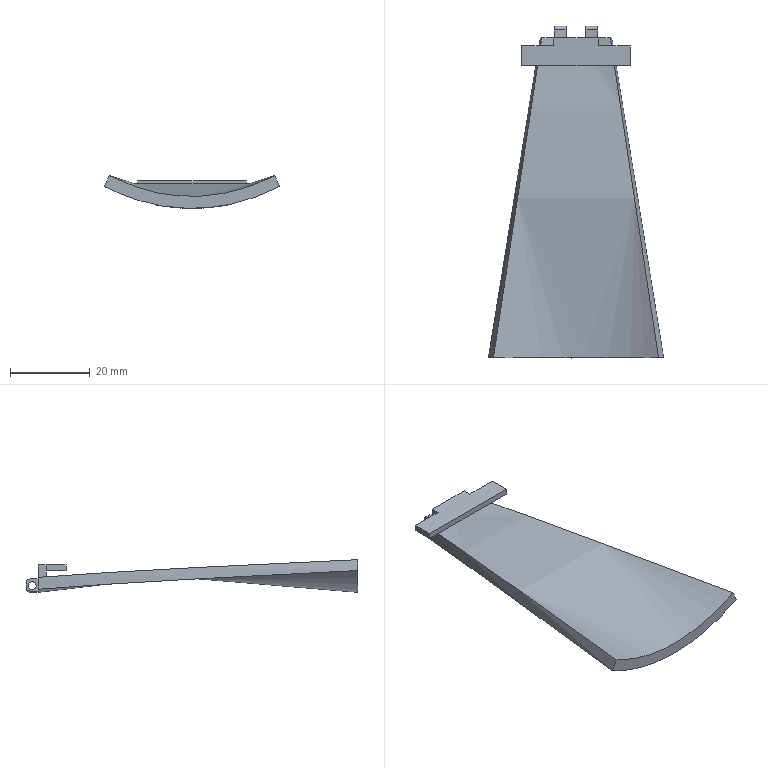Part | SolidWorks | features ICE 6, MoveFace 6, Blend 1, Fillet 1 | 1 solid | 34 faces | box 43.809 x 83 x 8.178 mm | volume 7265 mm3 | plane 18 | cylinder 8 | spline 4 | torus 4 | commonest cylinder face diameters 2 x4 86 x2 92 x2
STEP:
#1=CARTESIAN_POINT('',(-5.5,81.49,-43.311));
#2=VERTEX_POINT('',#1);
#3=CARTESIAN_POINT('',(-5.5,81.49,-45.311));
#4=VERTEX_POINT('',#3);
#5=CARTESIAN_POINT('',(-5.5,81.49,-44.311));
#6=DIRECTION('',(1.,0.,0.));
#7=DIRECTION('',(0.,0.,-1.));
#8=AXIS2_PLACEMENT_3D('',#5,#6,#7);
#9=CIRCLE('',#8,1.);
#10=EDGE_CURVE('',#2,#4,#9,.T.);
#11=ORIENTED_EDGE('',*,*,#10,.F.);
#12=CARTESIAN_POINT('',(-2.5,81.49,-43.311));
#13=VERTEX_POINT('',#12);
#14=CARTESIAN_POINT('',(-6.,81.49,-43.311));
#15=DIRECTION('',(1.,0.,0.));
#16=VECTOR('',#15,1000.);
#17=LINE('',#14,#16);
#18=EDGE_CURVE('',#2,#13,#17,.T.);
#19=ORIENTED_EDGE('',*,*,#18,.T.);
#20=CARTESIAN_POINT('',(-2.5,81.49,-45.311));
#21=VERTEX_POINT('',#20);
#22=CARTESIAN_POINT('',(-2.5,81.49,-44.311));
#23=DIRECTION('',(1.,0.,0.));
#24=DIRECTION('',(0.,0.,-1.));
#25=AXIS2_PLACEMENT_3D('',#22,#23,#24);
#26=CIRCLE('',#25,1.);
#27=EDGE_CURVE('',#13,#21,#26,.T.);
#28=ORIENTED_EDGE('',*,*,#27,.T.);
#29=CARTESIAN_POINT('',(-6.,81.49,-45.311));
#30=DIRECTION('',(1.,0.,0.));
#31=VECTOR('',#30,1000.);
#32=LINE('',#29,#31);
#33=EDGE_CURVE('',#4,#21,#32,.T.);
#34=ORIENTED_EDGE('',*,*,#33,.F.);
#35=EDGE_LOOP('',(#11,#19,#28,#34));
#36=FACE_OUTER_BOUND('',#35,.T.);
#37=CARTESIAN_POINT('',(-6.,81.49,-44.311));
#38=DIRECTION('',(1.,0.,0.));
#39=DIRECTION('',(0.,0.,-1.));
#40=AXIS2_PLACEMENT_3D('',#37,#38,#39);
#41=CYLINDRICAL_SURFACE('',#40,1.);
#42=ADVANCED_FACE('',(#36),#41,.F.);
#43=CARTESIAN_POINT('',(2.5,81.49,-45.311));
#44=VERTEX_POINT('',#43);
#45=CARTESIAN_POINT('',(2.5,81.49,-43.311));
#46=VERTEX_POINT('',#45);
#47=CARTESIAN_POINT('',(2.5,81.49,-44.311));
#48=DIRECTION('',(-1.,0.,0.));
#49=DIRECTION('',(0.,0.,1.));
#50=AXIS2_PLACEMENT_3D('',#47,#48,#49);
#51=CIRCLE('',#50,1.);
#52=EDGE_CURVE('',#44,#46,#51,.T.);
#53=ORIENTED_EDGE('',*,*,#52,.T.);
#54=CARTESIAN_POINT('',(5.5,81.49,-43.311));
#55=VERTEX_POINT('',#54);
#56=CARTESIAN_POINT('',(-6.,81.49,-43.311));
#57=DIRECTION('',(1.,0.,0.));
#58=VECTOR('',#57,1000.);
#59=LINE('',#56,#58);
#60=EDGE_CURVE('',#46,#55,#59,.T.);
#61=ORIENTED_EDGE('',*,*,#60,.T.);
#62=CARTESIAN_POINT('',(5.5,81.49,-45.311));
#63=VERTEX_POINT('',#62);
#64=CARTESIAN_POINT('',(5.5,81.49,-44.311));
#65=DIRECTION('',(1.,0.,0.));
#66=DIRECTION('',(0.,0.,-1.));
#67=AXIS2_PLACEMENT_3D('',#64,#65,#66);
#68=CIRCLE('',#67,1.);
#69=EDGE_CURVE('',#55,#63,#68,.T.);
#70=ORIENTED_EDGE('',*,*,#69,.T.);
#71=CARTESIAN_POINT('',(-6.,81.49,-45.311));
#72=DIRECTION('',(1.,0.,0.));
#73=VECTOR('',#72,1000.);
#74=LINE('',#71,#73);
#75=EDGE_CURVE('',#44,#63,#74,.T.);
#76=ORIENTED_EDGE('',*,*,#75,.F.);
#77=EDGE_LOOP('',(#53,#61,#70,#76));
#78=FACE_OUTER_BOUND('',#77,.T.);
#79=CARTESIAN_POINT('',(-6.,81.49,-44.311));
#80=DIRECTION('',(1.,0.,0.));
#81=DIRECTION('',(0.,0.,-1.));
#82=AXIS2_PLACEMENT_3D('',#79,#80,#81);
#83=CYLINDRICAL_SURFACE('',#82,1.);
#84=ADVANCED_FACE('',(#78),#83,.F.);
#85=CARTESIAN_POINT('',(-5.613,78.,-42.588));
#86=VERTEX_POINT('',#85);
#87=CARTESIAN_POINT('',(-5.613,78.,-40.632));
#88=VERTEX_POINT('',#87);
#89=CARTESIAN_POINT('',(-5.613,78.,-39.632));
#90=DIRECTION('',(0.,0.,1.));
#91=VECTOR('',#90,1000.);
#92=LINE('',#89,#91);
#93=EDGE_CURVE('',#86,#88,#92,.T.);
#94=ORIENTED_EDGE('',*,*,#93,.T.);
#95=CARTESIAN_POINT('',(-5.613,78.,-39.132));
#96=VERTEX_POINT('',#95);
#97=CARTESIAN_POINT('',(-5.613,78.,-38.132));
#98=DIRECTION('',(0.,0.,-1.));
#99=VECTOR('',#98,1000.);
#100=LINE('',#97,#99);
#101=EDGE_CURVE('',#96,#88,#100,.T.);
#102=ORIENTED_EDGE('',*,*,#101,.F.);
#103=CARTESIAN_POINT('',(-5.613,80.,-39.132));
#104=VERTEX_POINT('',#103);
#105=CARTESIAN_POINT('',(-5.613,78.,-39.132));
#106=DIRECTION('',(0.,1.,0.));
#107=VECTOR('',#106,1000.);
#108=LINE('',#105,#107);
#109=EDGE_CURVE('',#96,#104,#108,.T.);
#110=ORIENTED_EDGE('',*,*,#109,.T.);
#111=CARTESIAN_POINT('',(-5.613,80.,-42.632));
#112=VERTEX_POINT('',#111);
#113=CARTESIAN_POINT('',(-5.613,80.,-39.632));
#114=DIRECTION('',(0.,0.,1.));
#115=VECTOR('',#114,1000.);
#116=LINE('',#113,#115);
#117=EDGE_CURVE('',#112,#104,#116,.T.);
#118=ORIENTED_EDGE('',*,*,#117,.F.);
#119=CARTESIAN_POINT('',(-5.613,80.,-42.632));
#120=CARTESIAN_POINT('',(-5.613,79.333,-42.615));
#121=CARTESIAN_POINT('',(-5.613,78.667,-42.601));
#122=CARTESIAN_POINT('',(-5.613,78.,-42.588));
#123=B_SPLINE_CURVE_WITH_KNOTS('',3,(#119,#120,#121,#122),.UNSPECIFIED.,.F.,.F.,(4,4),(0.01005,0.01205),.UNSPECIFIED.);
#124=EDGE_CURVE('',#112,#86,#123,.T.);
#125=ORIENTED_EDGE('',*,*,#124,.T.);
#126=EDGE_LOOP('',(#94,#102,#110,#118,#125));
#127=FACE_OUTER_BOUND('',#126,.T.);
#128=CARTESIAN_POINT('',(-5.613,78.,-39.632));
#129=DIRECTION('',(-1.,0.,0.));
#130=DIRECTION('',(0.,0.,1.));
#131=AXIS2_PLACEMENT_3D('',#128,#129,#130);
#132=PLANE('',#131);
#133=ADVANCED_FACE('',(#127),#132,.T.);
#134=CARTESIAN_POINT('',(5.613,78.,-39.132));
#135=VERTEX_POINT('',#134);
#136=CARTESIAN_POINT('',(5.613,80.,-39.132));
#137=VERTEX_POINT('',#136);
#138=CARTESIAN_POINT('',(5.613,78.,-39.132));
#139=DIRECTION('',(0.,1.,0.));
#140=VECTOR('',#139,1000.);
#141=LINE('',#138,#140);
#142=EDGE_CURVE('',#135,#137,#141,.T.);
#143=ORIENTED_EDGE('',*,*,#142,.F.);
#144=CARTESIAN_POINT('',(5.613,78.,-40.632));
#145=VERTEX_POINT('',#144);
#146=CARTESIAN_POINT('',(5.613,78.,-38.132));
#147=DIRECTION('',(0.,0.,1.));
#148=VECTOR('',#147,1000.);
#149=LINE('',#146,#148);
#150=EDGE_CURVE('',#145,#135,#149,.T.);
#151=ORIENTED_EDGE('',*,*,#150,.F.);
#152=CARTESIAN_POINT('',(5.613,78.,-42.588));
#153=VERTEX_POINT('',#152);
#154=CARTESIAN_POINT('',(5.613,78.,-36.632));
#155=DIRECTION('',(0.,0.,-1.));
#156=VECTOR('',#155,1000.);
#157=LINE('',#154,#156);
#158=EDGE_CURVE('',#145,#153,#157,.T.);
#159=ORIENTED_EDGE('',*,*,#158,.T.);
#160=CARTESIAN_POINT('',(5.613,80.,-42.632));
#161=VERTEX_POINT('',#160);
#162=CARTESIAN_POINT('',(5.613,78.,-42.588));
#163=CARTESIAN_POINT('',(5.613,78.667,-42.601));
#164=CARTESIAN_POINT('',(5.613,79.333,-42.615));
#165=CARTESIAN_POINT('',(5.613,80.,-42.632));
#166=B_SPLINE_CURVE_WITH_KNOTS('',3,(#162,#163,#164,#165),.UNSPECIFIED.,.F.,.F.,(4,4),(0.01205,0.01405),.UNSPECIFIED.);
#167=EDGE_CURVE('',#153,#161,#166,.T.);
#168=ORIENTED_EDGE('',*,*,#167,.T.);
#169=CARTESIAN_POINT('',(5.613,80.,-36.632));
#170=DIRECTION('',(0.,0.,-1.));
#171=VECTOR('',#170,1000.);
#172=LINE('',#169,#171);
#173=EDGE_CURVE('',#137,#161,#172,.T.);
#174=ORIENTED_EDGE('',*,*,#173,.F.);
#175=EDGE_LOOP('',(#143,#151,#159,#168,#174));
#176=FACE_OUTER_BOUND('',#175,.T.);
#177=CARTESIAN_POINT('',(5.613,78.,-36.632));
#178=DIRECTION('',(1.,0.,0.));
#179=DIRECTION('',(0.,0.,-1.));
#180=AXIS2_PLACEMENT_3D('',#177,#178,#179);
#181=PLANE('',#180);
#182=ADVANCED_FACE('',(#176),#181,.T.);
#183=CARTESIAN_POINT('',(5.5,80.,-42.647));
#184=VERTEX_POINT('',#183);
#185=CARTESIAN_POINT('',(2.5,80.,-42.927));
#186=VERTEX_POINT('',#185);
#187=CARTESIAN_POINT('',(0.,80.,0.));
#188=DIRECTION('',(0.,1.,0.));
#189=DIRECTION('',(0.,0.,1.));
#190=AXIS2_PLACEMENT_3D('',#187,#188,#189);
#191=CIRCLE('',#190,43.);
#192=EDGE_CURVE('',#184,#186,#191,.T.);
#193=ORIENTED_EDGE('',*,*,#192,.T.);
#194=CARTESIAN_POINT('',(2.5,80.,-45.932));
#195=VERTEX_POINT('',#194);
#196=CARTESIAN_POINT('',(2.5,80.,0.));
#197=DIRECTION('',(0.,0.,-1.));
#198=VECTOR('',#197,1000.);
#199=LINE('',#196,#198);
#200=EDGE_CURVE('',#186,#195,#199,.T.);
#201=ORIENTED_EDGE('',*,*,#200,.T.);
#202=CARTESIAN_POINT('',(-2.5,80.,-45.932));
#203=VERTEX_POINT('',#202);
#204=CARTESIAN_POINT('',(0.,80.,0.));
#205=DIRECTION('',(0.,1.,0.));
#206=DIRECTION('',(0.,0.,-1.));
#207=AXIS2_PLACEMENT_3D('',#204,#205,#206);
#208=CIRCLE('',#207,46.);
#209=EDGE_CURVE('',#195,#203,#208,.T.);
#210=ORIENTED_EDGE('',*,*,#209,.T.);
#211=CARTESIAN_POINT('',(-2.5,80.,-42.927));
#212=VERTEX_POINT('',#211);
#213=CARTESIAN_POINT('',(-2.5,80.,0.));
#214=DIRECTION('',(0.,0.,1.));
#215=VECTOR('',#214,1000.);
#216=LINE('',#213,#215);
#217=EDGE_CURVE('',#203,#212,#216,.T.);
#218=ORIENTED_EDGE('',*,*,#217,.T.);
#219=CARTESIAN_POINT('',(-5.5,80.,-42.647));
#220=VERTEX_POINT('',#219);
#221=CARTESIAN_POINT('',(0.,80.,0.));
#222=DIRECTION('',(0.,-1.,0.));
#223=DIRECTION('',(0.,0.,1.));
#224=AXIS2_PLACEMENT_3D('',#221,#222,#223);
#225=CIRCLE('',#224,43.);
#226=EDGE_CURVE('',#220,#212,#225,.T.);
#227=ORIENTED_EDGE('',*,*,#226,.F.);
#228=CARTESIAN_POINT('',(-5.5,80.,-45.67));
#229=VERTEX_POINT('',#228);
#230=CARTESIAN_POINT('',(-5.5,80.,0.));
#231=DIRECTION('',(0.,0.,1.));
#232=VECTOR('',#231,1000.);
#233=LINE('',#230,#232);
#234=EDGE_CURVE('',#229,#220,#233,.T.);
#235=ORIENTED_EDGE('',*,*,#234,.F.);
#236=CARTESIAN_POINT('',(-8.953,80.,-45.218));
#237=VERTEX_POINT('',#236);
#238=CARTESIAN_POINT('',(-5.5,80.,-45.67));
#239=CARTESIAN_POINT('',(-5.788,80.,-45.635));
#240=CARTESIAN_POINT('',(-6.076,80.,-45.597));
#241=CARTESIAN_POINT('',(-6.651,80.,-45.521));
#242=CARTESIAN_POINT('',(-7.515,80.,-45.408));
#243=CARTESIAN_POINT('',(-8.378,80.,-45.294));
#244=CARTESIAN_POINT('',(-8.953,80.,-45.218));
#245=B_SPLINE_CURVE_WITH_KNOTS('',3,(#238,#239,#240,#241,#242,#243,#244),.UNSPECIFIED.,.F.,.F.,(4,2,1,4),(0.,0.0008706,0.001741,0.003483),.UNSPECIFIED.);
#246=EDGE_CURVE('',#229,#237,#245,.T.);
#247=ORIENTED_EDGE('',*,*,#246,.T.);
#248=CARTESIAN_POINT('',(-8.562,80.,-42.244));
#249=VERTEX_POINT('',#248);
#250=CARTESIAN_POINT('',(-8.953,80.,-45.218));
#251=CARTESIAN_POINT('',(-8.823,80.,-44.227));
#252=CARTESIAN_POINT('',(-8.692,80.,-43.235));
#253=CARTESIAN_POINT('',(-8.562,80.,-42.244));
#254=B_SPLINE_CURVE_WITH_KNOTS('',3,(#250,#251,#252,#253),.UNSPECIFIED.,.F.,.F.,(4,4),(0.,1.),.UNSPECIFIED.);
#255=EDGE_CURVE('',#237,#249,#254,.T.);
#256=ORIENTED_EDGE('',*,*,#255,.T.);
#257=CARTESIAN_POINT('',(-5.613,80.,-42.632));
#258=CARTESIAN_POINT('',(-6.596,80.,-42.503));
#259=CARTESIAN_POINT('',(-7.579,80.,-42.373));
#260=CARTESIAN_POINT('',(-8.562,80.,-42.244));
#261=B_SPLINE_CURVE_WITH_KNOTS('',3,(#257,#258,#259,#260),.UNSPECIFIED.,.F.,.F.,(4,4),(0.,0.002974),.UNSPECIFIED.);
#262=EDGE_CURVE('',#112,#249,#261,.T.);
#263=ORIENTED_EDGE('',*,*,#262,.F.);
#264=ORIENTED_EDGE('',*,*,#117,.T.);
#265=CARTESIAN_POINT('',(-5.613,80.,-39.132));
#266=DIRECTION('',(1.,0.,0.));
#267=VECTOR('',#266,1000.);
#268=LINE('',#265,#267);
#269=EDGE_CURVE('',#104,#137,#268,.T.);
#270=ORIENTED_EDGE('',*,*,#269,.T.);
#271=ORIENTED_EDGE('',*,*,#173,.T.);
#272=CARTESIAN_POINT('',(8.562,80.,-42.244));
#273=VERTEX_POINT('',#272);
#274=CARTESIAN_POINT('',(5.613,80.,-42.632));
#275=CARTESIAN_POINT('',(6.596,80.,-42.503));
#276=CARTESIAN_POINT('',(7.579,80.,-42.373));
#277=CARTESIAN_POINT('',(8.562,80.,-42.244));
#278=B_SPLINE_CURVE_WITH_KNOTS('',3,(#274,#275,#276,#277),.UNSPECIFIED.,.F.,.F.,(4,4),(0.,0.002974),.UNSPECIFIED.);
#279=EDGE_CURVE('',#161,#273,#278,.T.);
#280=ORIENTED_EDGE('',*,*,#279,.T.);
#281=CARTESIAN_POINT('',(8.953,80.,-45.218));
#282=VERTEX_POINT('',#281);
#283=CARTESIAN_POINT('',(8.562,80.,-42.244));
#284=CARTESIAN_POINT('',(8.692,80.,-43.235));
#285=CARTESIAN_POINT('',(8.823,80.,-44.227));
#286=CARTESIAN_POINT('',(8.953,80.,-45.218));
#287=B_SPLINE_CURVE_WITH_KNOTS('',3,(#283,#284,#285,#286),.UNSPECIFIED.,.F.,.F.,(4,4),(0.,1.),.UNSPECIFIED.);
#288=EDGE_CURVE('',#273,#282,#287,.T.);
#289=ORIENTED_EDGE('',*,*,#288,.T.);
#290=CARTESIAN_POINT('',(5.5,80.,-45.67));
#291=VERTEX_POINT('',#290);
#292=CARTESIAN_POINT('',(8.953,80.,-45.218));
#293=CARTESIAN_POINT('',(8.378,80.,-45.294));
#294=CARTESIAN_POINT('',(7.515,80.,-45.408));
#295=CARTESIAN_POINT('',(6.651,80.,-45.521));
#296=CARTESIAN_POINT('',(6.076,80.,-45.597));
#297=CARTESIAN_POINT('',(5.788,80.,-45.635));
#298=CARTESIAN_POINT('',(5.5,80.,-45.67));
#299=B_SPLINE_CURVE_WITH_KNOTS('',3,(#292,#293,#294,#295,#296,#297,#298),.UNSPECIFIED.,.F.,.F.,(4,1,2,4),(0.,0.001741,0.002612,0.003483),.UNSPECIFIED.);
#300=EDGE_CURVE('',#282,#291,#299,.T.);
#301=ORIENTED_EDGE('',*,*,#300,.T.);
#302=CARTESIAN_POINT('',(5.5,80.,0.));
#303=DIRECTION('',(0.,0.,1.));
#304=VECTOR('',#303,1000.);
#305=LINE('',#302,#304);
#306=EDGE_CURVE('',#291,#184,#305,.T.);
#307=ORIENTED_EDGE('',*,*,#306,.T.);
#308=EDGE_LOOP('',(#193,#201,#210,#218,#227,#235,#247,#256,#263,#264,#270,#271,#280,#289,#301,#307));
#309=FACE_OUTER_BOUND('',#308,.T.);
#310=CARTESIAN_POINT('',(0.,80.,0.));
#311=DIRECTION('',(0.,-1.,0.));
#312=DIRECTION('',(0.,0.,-1.));
#313=AXIS2_PLACEMENT_3D('',#310,#311,#312);
#314=PLANE('',#313);
#315=ADVANCED_FACE('',(#309),#314,.F.);
#316=ORIENTED_EDGE('',*,*,#158,.F.);
#317=CARTESIAN_POINT('',(-5.613,78.,-40.632));
#318=DIRECTION('',(1.,0.,0.));
#319=VECTOR('',#318,1000.);
#320=LINE('',#317,#319);
#321=EDGE_CURVE('',#88,#145,#320,.T.);
#322=ORIENTED_EDGE('',*,*,#321,.F.);
#323=ORIENTED_EDGE('',*,*,#93,.F.);
#324=CARTESIAN_POINT('',(-5.613,78.,-42.588));
#325=CARTESIAN_POINT('',(-3.752,78.,-42.862));
#326=CARTESIAN_POINT('',(-1.88,78.,-43.));
#327=CARTESIAN_POINT('',(1.881,78.,-43.));
#328=CARTESIAN_POINT('',(3.752,78.,-42.862));
#329=CARTESIAN_POINT('',(5.613,78.,-42.588));
#330=B_SPLINE_CURVE_WITH_KNOTS('',3,(#324,#325,#326,#327,#328,#329),.UNSPECIFIED.,.F.,.F.,(4,2,4),(0.,0.005628,0.01126),.UNSPECIFIED.);
#331=EDGE_CURVE('',#86,#153,#330,.T.);
#332=ORIENTED_EDGE('',*,*,#331,.T.);
#333=EDGE_LOOP('',(#316,#322,#323,#332));
#334=FACE_OUTER_BOUND('',#333,.T.);
#335=CARTESIAN_POINT('',(0.,78.,3.));
#336=DIRECTION('',(0.,-1.,0.));
#337=DIRECTION('',(0.,0.,-1.));
#338=AXIS2_PLACEMENT_3D('',#335,#336,#337);
#339=PLANE('',#338);
#340=ADVANCED_FACE('',(#334),#339,.T.);
#341=CARTESIAN_POINT('',(21.905,0.,-40.541));
#342=VERTEX_POINT('',#341);
#343=CARTESIAN_POINT('',(-21.905,0.,-40.541));
#344=VERTEX_POINT('',#343);
#345=CARTESIAN_POINT('',(21.905,0.,-40.541));
#346=CARTESIAN_POINT('',(21.068,0.,-40.931));
#347=CARTESIAN_POINT('',(20.232,0.,-41.322));
#348=CARTESIAN_POINT('',(18.557,0.,-42.101));
#349=CARTESIAN_POINT('',(17.702,0.,-42.468));
#350=CARTESIAN_POINT('',(15.091,0.,-43.494));
#351=CARTESIAN_POINT('',(13.289,0.,-44.08));
#352=CARTESIAN_POINT('',(9.595,0.,-45.029));
#353=CARTESIAN_POINT('',(7.703,0.,-45.391));
#354=CARTESIAN_POINT('',(3.875,0.,-45.877));
#355=CARTESIAN_POINT('',(1.937,0.,-46.));
#356=CARTESIAN_POINT('',(-1.937,0.,-46.));
#357=CARTESIAN_POINT('',(-3.875,0.,-45.877));
#358=CARTESIAN_POINT('',(-7.703,0.,-45.391));
#359=CARTESIAN_POINT('',(-9.595,0.,-45.029));
#360=CARTESIAN_POINT('',(-13.289,0.,-44.08));
#361=CARTESIAN_POINT('',(-15.091,0.,-43.494));
#362=CARTESIAN_POINT('',(-17.702,0.,-42.468));
#363=CARTESIAN_POINT('',(-18.557,0.,-42.101));
#364=CARTESIAN_POINT('',(-20.232,0.,-41.322));
#365=CARTESIAN_POINT('',(-21.068,0.,-40.931));
#366=CARTESIAN_POINT('',(-21.905,0.,-40.541));
#367=B_SPLINE_CURVE_WITH_KNOTS('',3,(#345,#346,#347,#348,#349,#350,#351,#352,#353,#354,#355,#356,#357,#358,#359,#360,#361,#362,#363,#364,#365,#366),.UNSPECIFIED.,.F.,.F.,(4,2,2,2,2,2,2,2,2,2,4),(0.,0.002828,0.005655,0.01131,0.01697,0.02262,0.02828,0.03393,0.03959,0.04242,0.04524),.UNSPECIFIED.);
#368=EDGE_CURVE('',#342,#344,#367,.T.);
#369=ORIENTED_EDGE('',*,*,#368,.F.);
#370=CARTESIAN_POINT('',(20.637,0.,-37.822));
#371=VERTEX_POINT('',#370);
#372=CARTESIAN_POINT('',(20.637,0.,-37.822));
#373=CARTESIAN_POINT('',(20.76,0.,-38.087));
#374=CARTESIAN_POINT('',(20.884,0.,-38.352));
#375=CARTESIAN_POINT('',(21.007,0.,-38.616));
#376=CARTESIAN_POINT('',(21.062,0.,-38.735));
#377=CARTESIAN_POINT('',(21.117,0.,-38.853));
#378=CARTESIAN_POINT('',(21.173,0.,-38.971));
#379=CARTESIAN_POINT('',(21.384,0.,-39.424));
#380=CARTESIAN_POINT('',(21.595,0.,-39.878));
#381=CARTESIAN_POINT('',(21.839,0.,-40.401));
#382=CARTESIAN_POINT('',(21.872,0.,-40.471));
#383=CARTESIAN_POINT('',(21.905,0.,-40.541));
#384=B_SPLINE_CURVE_WITH_KNOTS('',3,(#372,#373,#374,#375,#376,#377,#378,#379,#380,#381,#382,#383),.UNSPECIFIED.,.F.,.F.,(4,3,3,2,4),(-0.4226,-0.1305,0.,0.5,0.5774),.UNSPECIFIED.);
#385=EDGE_CURVE('',#371,#342,#384,.T.);
#386=ORIENTED_EDGE('',*,*,#385,.F.);
#387=CARTESIAN_POINT('',(-20.637,0.,-37.822));
#388=VERTEX_POINT('',#387);
#389=CARTESIAN_POINT('',(-20.637,0.,-37.822));
#390=CARTESIAN_POINT('',(-19.848,0.,-38.19));
#391=CARTESIAN_POINT('',(-19.059,0.,-38.558));
#392=CARTESIAN_POINT('',(-17.481,0.,-39.294));
#393=CARTESIAN_POINT('',(-16.678,0.,-39.644));
#394=CARTESIAN_POINT('',(-14.221,0.,-40.618));
#395=CARTESIAN_POINT('',(-12.524,0.,-41.175));
#396=CARTESIAN_POINT('',(-9.044,0.,-42.077));
#397=CARTESIAN_POINT('',(-7.262,0.,-42.421));
#398=CARTESIAN_POINT('',(-3.653,0.,-42.883));
#399=CARTESIAN_POINT('',(-1.827,0.,-43.));
#400=CARTESIAN_POINT('',(1.827,0.,-43.));
#401=CARTESIAN_POINT('',(3.653,0.,-42.883));
#402=CARTESIAN_POINT('',(7.262,0.,-42.421));
#403=CARTESIAN_POINT('',(9.044,0.,-42.077));
#404=CARTESIAN_POINT('',(12.524,0.,-41.175));
#405=CARTESIAN_POINT('',(14.221,0.,-40.618));
#406=CARTESIAN_POINT('',(16.678,0.,-39.644));
#407=CARTESIAN_POINT('',(17.481,0.,-39.294));
#408=CARTESIAN_POINT('',(19.059,0.,-38.558));
#409=CARTESIAN_POINT('',(19.848,0.,-38.19));
#410=CARTESIAN_POINT('',(20.637,0.,-37.822));
#411=B_SPLINE_CURVE_WITH_KNOTS('',3,(#389,#390,#391,#392,#393,#394,#395,#396,#397,#398,#399,#400,#401,#402,#403,#404,#405,#406,#407,#408,#409,#410),.UNSPECIFIED.,.F.,.F.,(4,2,2,2,2,2,2,2,2,2,4),(-0.002673,-0.00001107,0.002651,0.007976,0.0133,0.01862,0.02395,0.02927,0.0346,0.03726,0.03992),.UNSPECIFIED.);
#412=EDGE_CURVE('',#388,#371,#411,.T.);
#413=ORIENTED_EDGE('',*,*,#412,.F.);
#414=CARTESIAN_POINT('',(-21.905,0.,-40.541));
#415=CARTESIAN_POINT('',(-21.872,0.,-40.471));
#416=CARTESIAN_POINT('',(-21.839,0.,-40.401));
#417=CARTESIAN_POINT('',(-21.595,0.,-39.878));
#418=CARTESIAN_POINT('',(-21.384,0.,-39.424));
#419=CARTESIAN_POINT('',(-21.173,0.,-38.971));
#420=CARTESIAN_POINT('',(-21.117,0.,-38.853));
#421=CARTESIAN_POINT('',(-21.062,0.,-38.735));
#422=CARTESIAN_POINT('',(-21.007,0.,-38.616));
#423=CARTESIAN_POINT('',(-20.884,0.,-38.352));
#424=CARTESIAN_POINT('',(-20.76,0.,-38.087));
#425=CARTESIAN_POINT('',(-20.637,0.,-37.822));
#426=B_SPLINE_CURVE_WITH_KNOTS('',3,(#414,#415,#416,#417,#418,#419,#420,#421,#422,#423,#424,#425),.UNSPECIFIED.,.F.,.F.,(4,2,3,3,4),(0.4226,0.5,1.,1.131,1.423),.UNSPECIFIED.);
#427=EDGE_CURVE('',#344,#388,#426,.T.);
#428=ORIENTED_EDGE('',*,*,#427,.F.);
#429=EDGE_LOOP('',(#369,#386,#413,#428));
#430=FACE_OUTER_BOUND('',#429,.T.);
#431=CARTESIAN_POINT('',(0.,0.,0.));
#432=DIRECTION('',(0.,-1.,0.));
#433=DIRECTION('',(0.,0.,-1.));
#434=AXIS2_PLACEMENT_3D('',#431,#432,#433);
#435=PLANE('',#434);
#436=ADVANCED_FACE('',(#430),#435,.T.);
#437=ORIENTED_EDGE('',*,*,#288,.F.);
#438=CARTESIAN_POINT('',(8.562,80.,-42.244));
#439=CARTESIAN_POINT('',(9.064,76.672,-41.978));
#440=CARTESIAN_POINT('',(9.566,73.342,-41.739));
#441=CARTESIAN_POINT('',(10.571,66.68,-41.291));
#442=CARTESIAN_POINT('',(11.073,63.347,-41.083));
#443=CARTESIAN_POINT('',(12.58,53.349,-40.485));
#444=CARTESIAN_POINT('',(13.585,46.682,-40.122));
#445=CARTESIAN_POINT('',(15.597,33.346,-39.428));
#446=CARTESIAN_POINT('',(16.604,26.677,-39.096));
#447=CARTESIAN_POINT('',(18.619,13.339,-38.449));
#448=CARTESIAN_POINT('',(19.627,6.669,-38.133));
#449=CARTESIAN_POINT('',(20.637,0.,-37.822));
#450=B_SPLINE_CURVE_WITH_KNOTS('',3,(#438,#439,#440,#441,#442,#443,#444,#445,#446,#447,#448,#449),.UNSPECIFIED.,.F.,.F.,(4,2,2,2,2,4),(0.3445,0.3546,0.3647,0.385,0.4052,0.4255),.UNSPECIFIED.);
#451=EDGE_CURVE('',#273,#371,#450,.T.);
#452=ORIENTED_EDGE('',*,*,#451,.T.);
#453=ORIENTED_EDGE('',*,*,#385,.T.);
#454=CARTESIAN_POINT('',(21.905,0.,-40.541));
#455=CARTESIAN_POINT('',(20.822,6.67,-40.873));
#456=CARTESIAN_POINT('',(19.741,13.339,-41.21));
#457=CARTESIAN_POINT('',(17.579,26.677,-41.9));
#458=CARTESIAN_POINT('',(16.499,33.346,-42.253));
#459=CARTESIAN_POINT('',(14.341,46.683,-42.99));
#460=CARTESIAN_POINT('',(13.263,53.35,-43.374));
#461=CARTESIAN_POINT('',(11.647,63.348,-44.003));
#462=CARTESIAN_POINT('',(11.108,66.68,-44.222));
#463=CARTESIAN_POINT('',(10.031,73.342,-44.692));
#464=CARTESIAN_POINT('',(9.492,76.672,-44.941));
#465=CARTESIAN_POINT('',(8.953,80.,-45.218));
#466=B_SPLINE_CURVE_WITH_KNOTS('',3,(#454,#455,#456,#457,#458,#459,#460,#461,#462,#463,#464,#465),.UNSPECIFIED.,.F.,.F.,(4,2,2,2,2,4),(0.,0.02029,0.04059,0.06088,0.07103,0.08118),.UNSPECIFIED.);
#467=EDGE_CURVE('',#342,#282,#466,.T.);
#468=ORIENTED_EDGE('',*,*,#467,.T.);
#469=EDGE_LOOP('',(#437,#452,#453,#468));
#470=FACE_OUTER_BOUND('',#469,.T.);
#471=CARTESIAN_POINT('',(9.004,80.,-45.606));
#472=CARTESIAN_POINT('',(22.44,0.,-41.69));
#473=CARTESIAN_POINT('',(8.939,80.,-45.111));
#474=CARTESIAN_POINT('',(22.229,0.,-41.237));
#475=CARTESIAN_POINT('',(8.874,80.,-44.615));
#476=CARTESIAN_POINT('',(22.018,0.,-40.784));
#477=CARTESIAN_POINT('',(8.743,80.,-43.624));
#478=CARTESIAN_POINT('',(21.595,0.,-39.878));
#479=CARTESIAN_POINT('',(8.678,80.,-43.128));
#480=CARTESIAN_POINT('',(21.384,0.,-39.424));
#481=CARTESIAN_POINT('',(8.613,80.,-42.632));
#482=CARTESIAN_POINT('',(21.173,0.,-38.971));
#483=CARTESIAN_POINT('',(8.596,80.,-42.503));
#484=CARTESIAN_POINT('',(21.117,0.,-38.853));
#485=CARTESIAN_POINT('',(8.579,80.,-42.373));
#486=CARTESIAN_POINT('',(21.062,0.,-38.735));
#487=CARTESIAN_POINT('',(8.562,80.,-42.244));
#488=CARTESIAN_POINT('',(21.007,0.,-38.616));
#489=CARTESIAN_POINT('',(8.523,80.,-41.954));
#490=CARTESIAN_POINT('',(20.884,0.,-38.352));
#491=CARTESIAN_POINT('',(8.485,80.,-41.665));
#492=CARTESIAN_POINT('',(20.76,0.,-38.087));
#493=CARTESIAN_POINT('',(8.447,80.,-41.375));
#494=CARTESIAN_POINT('',(20.637,0.,-37.822));
#495=B_SPLINE_SURFACE_WITH_KNOTS('',3,1,((#471,#472),(#473,#474),(#475,#476),(#477,#478),(#479,#480),(#481,#482),(#483,#484),(#485,#486),(#487,#488),(#489,#490),(#491,#492),(#493,#494)),.UNSPECIFIED.,.F.,.F.,.F.,(4,2,3,3,4),(2,2),(0.,0.5,1.,1.131,1.423),(0.,1.),.UNSPECIFIED.);
#496=ADVANCED_FACE('',(#470),#495,.T.);
#497=ORIENTED_EDGE('',*,*,#167,.F.);
#498=ORIENTED_EDGE('',*,*,#331,.F.);
#499=ORIENTED_EDGE('',*,*,#124,.F.);
#500=ORIENTED_EDGE('',*,*,#262,.T.);
#501=CARTESIAN_POINT('',(-8.562,80.,-42.244));
#502=CARTESIAN_POINT('',(-9.064,76.672,-41.978));
#503=CARTESIAN_POINT('',(-9.566,73.342,-41.739));
#504=CARTESIAN_POINT('',(-10.571,66.68,-41.291));
#505=CARTESIAN_POINT('',(-11.073,63.347,-41.083));
#506=CARTESIAN_POINT('',(-12.58,53.349,-40.485));
#507=CARTESIAN_POINT('',(-13.585,46.682,-40.122));
#508=CARTESIAN_POINT('',(-15.597,33.346,-39.428));
#509=CARTESIAN_POINT('',(-16.604,26.677,-39.096));
#510=CARTESIAN_POINT('',(-18.619,13.339,-38.449));
#511=CARTESIAN_POINT('',(-19.627,6.669,-38.133));
#512=CARTESIAN_POINT('',(-20.637,0.,-37.822));
#513=B_SPLINE_CURVE_WITH_KNOTS('',3,(#501,#502,#503,#504,#505,#506,#507,#508,#509,#510,#511,#512),.UNSPECIFIED.,.F.,.F.,(4,2,2,2,2,4),(0.339,0.3491,0.3592,0.3795,0.3997,0.42),.UNSPECIFIED.);
#514=EDGE_CURVE('',#249,#388,#513,.T.);
#515=ORIENTED_EDGE('',*,*,#514,.T.);
#516=ORIENTED_EDGE('',*,*,#412,.T.);
#517=ORIENTED_EDGE('',*,*,#451,.F.);
#518=ORIENTED_EDGE('',*,*,#279,.F.);
#519=EDGE_LOOP('',(#497,#498,#499,#500,#515,#516,#517,#518));
#520=FACE_OUTER_BOUND('',#519,.T.);
#521=CARTESIAN_POINT('',(5.613,80.,-42.632));
#522=CARTESIAN_POINT('',(18.173,0.,-38.971));
#523=CARTESIAN_POINT('',(1.882,80.,-43.123));
#524=CARTESIAN_POINT('',(6.461,0.,-44.432));
#525=CARTESIAN_POINT('',(-1.882,80.,-43.123));
#526=CARTESIAN_POINT('',(-6.461,0.,-44.432));
#527=CARTESIAN_POINT('',(-5.613,80.,-42.632));
#528=CARTESIAN_POINT('',(-18.173,0.,-38.971));
#529=(BOUNDED_SURFACE()B_SPLINE_SURFACE(3,1,((#521,#522),(#523,#524),(#525,#526),(#527,#528)),.UNSPECIFIED.,.F.,.F.,.F.)B_SPLINE_SURFACE_WITH_KNOTS((4,4),(2,2),(0.,1.),(0.,1.),.UNSPECIFIED.)GEOMETRIC_REPRESENTATION_ITEM()RATIONAL_B_SPLINE_SURFACE(((1.,1.),(0.9943,0.9375),(0.9943,0.9375),(1.,1.)))REPRESENTATION_ITEM('')SURFACE());
#530=ADVANCED_FACE('',(#520),#529,.T.);
#531=ORIENTED_EDGE('',*,*,#300,.F.);
#532=ORIENTED_EDGE('',*,*,#467,.F.);
#533=ORIENTED_EDGE('',*,*,#368,.T.);
#534=CARTESIAN_POINT('',(-8.953,80.,-45.218));
#535=CARTESIAN_POINT('',(-9.492,76.672,-44.941));
#536=CARTESIAN_POINT('',(-10.031,73.342,-44.692));
#537=CARTESIAN_POINT('',(-11.108,66.68,-44.222));
#538=CARTESIAN_POINT('',(-11.647,63.348,-44.003));
#539=CARTESIAN_POINT('',(-13.263,53.35,-43.374));
#540=CARTESIAN_POINT('',(-14.341,46.682,-42.99));
#541=CARTESIAN_POINT('',(-16.499,33.346,-42.253));
#542=CARTESIAN_POINT('',(-17.579,26.677,-41.9));
#543=CARTESIAN_POINT('',(-19.741,13.339,-41.21));
#544=CARTESIAN_POINT('',(-20.822,6.67,-40.873));
#545=CARTESIAN_POINT('',(-21.905,0.,-40.541));
#546=B_SPLINE_CURVE_WITH_KNOTS('',3,(#534,#535,#536,#537,#538,#539,#540,#541,#542,#543,#544,#545),.UNSPECIFIED.,.F.,.F.,(4,2,2,2,2,4),(0.,0.01015,0.0203,0.04059,0.06089,0.08118),.UNSPECIFIED.);
#547=EDGE_CURVE('',#237,#344,#546,.T.);
#548=ORIENTED_EDGE('',*,*,#547,.F.);
#549=ORIENTED_EDGE('',*,*,#246,.F.);
#550=CARTESIAN_POINT('',(0.,80.,0.));
#551=DIRECTION('',(0.,1.,0.));
#552=DIRECTION('',(0.,0.,-1.));
#553=AXIS2_PLACEMENT_3D('',#550,#551,#552);
#554=CIRCLE('',#553,46.);
#555=EDGE_CURVE('',#203,#229,#554,.T.);
#556=ORIENTED_EDGE('',*,*,#555,.F.);
#557=ORIENTED_EDGE('',*,*,#209,.F.);
#558=CARTESIAN_POINT('',(0.,80.,0.));
#559=DIRECTION('',(0.,1.,0.));
#560=DIRECTION('',(0.,0.,-1.));
#561=AXIS2_PLACEMENT_3D('',#558,#559,#560);
#562=CIRCLE('',#561,46.);
#563=EDGE_CURVE('',#291,#195,#562,.T.);
#564=ORIENTED_EDGE('',*,*,#563,.F.);
#565=EDGE_LOOP('',(#531,#532,#533,#548,#549,#556,#557,#564));
#566=FACE_OUTER_BOUND('',#565,.T.);
#567=CARTESIAN_POINT('',(-6.004,80.,-45.606));
#568=CARTESIAN_POINT('',(-19.44,0.,-41.69));
#569=CARTESIAN_POINT('',(-2.013,80.,-46.132));
#570=CARTESIAN_POINT('',(-6.912,0.,-47.532));
#571=CARTESIAN_POINT('',(2.013,80.,-46.132));
#572=CARTESIAN_POINT('',(6.912,0.,-47.532));
#573=CARTESIAN_POINT('',(6.004,80.,-45.606));
#574=CARTESIAN_POINT('',(19.44,0.,-41.69));
#575=(BOUNDED_SURFACE()B_SPLINE_SURFACE(3,1,((#567,#568),(#569,#570),(#571,#572),(#573,#574)),.UNSPECIFIED.,.F.,.F.,.F.)B_SPLINE_SURFACE_WITH_KNOTS((4,4),(2,2),(0.,1.),(0.,1.),.UNSPECIFIED.)GEOMETRIC_REPRESENTATION_ITEM()RATIONAL_B_SPLINE_SURFACE(((1.,1.),(0.9943,0.9375),(0.9943,0.9375),(1.,1.)))REPRESENTATION_ITEM('')SURFACE());
#576=ADVANCED_FACE('',(#566),#575,.T.);
#577=ORIENTED_EDGE('',*,*,#255,.F.);
#578=ORIENTED_EDGE('',*,*,#547,.T.);
#579=ORIENTED_EDGE('',*,*,#427,.T.);
#580=ORIENTED_EDGE('',*,*,#514,.F.);
#581=EDGE_LOOP('',(#577,#578,#579,#580));
#582=FACE_OUTER_BOUND('',#581,.T.);
#583=CARTESIAN_POINT('',(-8.447,80.,-41.375));
#584=CARTESIAN_POINT('',(-20.637,0.,-37.822));
#585=CARTESIAN_POINT('',(-8.485,80.,-41.665));
#586=CARTESIAN_POINT('',(-20.76,0.,-38.087));
#587=CARTESIAN_POINT('',(-8.523,80.,-41.954));
#588=CARTESIAN_POINT('',(-20.884,0.,-38.352));
#589=CARTESIAN_POINT('',(-8.562,80.,-42.244));
#590=CARTESIAN_POINT('',(-21.007,0.,-38.616));
#591=CARTESIAN_POINT('',(-8.579,80.,-42.373));
#592=CARTESIAN_POINT('',(-21.062,0.,-38.735));
#593=CARTESIAN_POINT('',(-8.596,80.,-42.503));
#594=CARTESIAN_POINT('',(-21.117,0.,-38.853));
#595=CARTESIAN_POINT('',(-8.613,80.,-42.632));
#596=CARTESIAN_POINT('',(-21.173,0.,-38.971));
#597=CARTESIAN_POINT('',(-8.678,80.,-43.128));
#598=CARTESIAN_POINT('',(-21.384,0.,-39.424));
#599=CARTESIAN_POINT('',(-8.743,80.,-43.624));
#600=CARTESIAN_POINT('',(-21.595,0.,-39.878));
#601=CARTESIAN_POINT('',(-8.874,80.,-44.615));
#602=CARTESIAN_POINT('',(-22.018,0.,-40.784));
#603=CARTESIAN_POINT('',(-8.939,80.,-45.111));
#604=CARTESIAN_POINT('',(-22.229,0.,-41.237));
#605=CARTESIAN_POINT('',(-9.004,80.,-45.606));
#606=CARTESIAN_POINT('',(-22.44,0.,-41.69));
#607=B_SPLINE_SURFACE_WITH_KNOTS('',3,1,((#583,#584),(#585,#586),(#587,#588),(#589,#590),(#591,#592),(#593,#594),(#595,#596),(#597,#598),(#599,#600),(#601,#602),(#603,#604),(#605,#606)),.UNSPECIFIED.,.F.,.F.,.F.,(4,3,3,2,4),(2,2),(-0.4226,-0.1305,0.,0.5,1.),(0.,1.),.UNSPECIFIED.);
#608=ADVANCED_FACE('',(#582),#607,.T.);
#609=ORIENTED_EDGE('',*,*,#269,.F.);
#610=ORIENTED_EDGE('',*,*,#109,.F.);
#611=CARTESIAN_POINT('',(-13.613,78.,-39.132));
#612=VERTEX_POINT('',#611);
#613=CARTESIAN_POINT('',(-10.613,78.,-39.132));
#614=DIRECTION('',(1.,0.,0.));
#615=VECTOR('',#614,1000.);
#616=LINE('',#613,#615);
#617=EDGE_CURVE('',#612,#96,#616,.T.);
#618=ORIENTED_EDGE('',*,*,#617,.F.);
#619=CARTESIAN_POINT('',(-13.613,73.,-39.132));
#620=VERTEX_POINT('',#619);
#621=CARTESIAN_POINT('',(-13.613,78.,-39.132));
#622=DIRECTION('',(0.,1.,0.));
#623=VECTOR('',#622,1000.);
#624=LINE('',#621,#623);
#625=EDGE_CURVE('',#620,#612,#624,.T.);
#626=ORIENTED_EDGE('',*,*,#625,.F.);
#627=CARTESIAN_POINT('',(13.613,73.,-39.132));
#628=VERTEX_POINT('',#627);
#629=CARTESIAN_POINT('',(-5.613,73.,-39.132));
#630=DIRECTION('',(-1.,0.,0.));
#631=VECTOR('',#630,1000.);
#632=LINE('',#629,#631);
#633=EDGE_CURVE('',#628,#620,#632,.T.);
#634=ORIENTED_EDGE('',*,*,#633,.F.);
#635=CARTESIAN_POINT('',(13.613,78.,-39.132));
#636=VERTEX_POINT('',#635);
#637=CARTESIAN_POINT('',(13.613,78.,-39.132));
#638=DIRECTION('',(0.,-1.,0.));
#639=VECTOR('',#638,1000.);
#640=LINE('',#637,#639);
#641=EDGE_CURVE('',#636,#628,#640,.T.);
#642=ORIENTED_EDGE('',*,*,#641,.F.);
#643=CARTESIAN_POINT('',(10.613,78.,-39.132));
#644=DIRECTION('',(-1.,0.,0.));
#645=VECTOR('',#644,1000.);
#646=LINE('',#643,#645);
#647=EDGE_CURVE('',#636,#135,#646,.T.);
#648=ORIENTED_EDGE('',*,*,#647,.T.);
#649=ORIENTED_EDGE('',*,*,#142,.T.);
#650=EDGE_LOOP('',(#609,#610,#618,#626,#634,#642,#648,#649));
#651=FACE_OUTER_BOUND('',#650,.T.);
#652=CARTESIAN_POINT('',(-5.613,78.,-39.132));
#653=DIRECTION('',(0.,0.,1.));
#654=DIRECTION('',(1.,0.,0.));
#655=AXIS2_PLACEMENT_3D('',#652,#653,#654);
#656=PLANE('',#655);
#657=ADVANCED_FACE('',(#651),#656,.T.);
#658=ORIENTED_EDGE('',*,*,#321,.T.);
#659=CARTESIAN_POINT('',(13.613,78.,-40.632));
#660=VERTEX_POINT('',#659);
#661=CARTESIAN_POINT('',(10.613,78.,-40.632));
#662=DIRECTION('',(-1.,0.,0.));
#663=VECTOR('',#662,1000.);
#664=LINE('',#661,#663);
#665=EDGE_CURVE('',#660,#145,#664,.T.);
#666=ORIENTED_EDGE('',*,*,#665,.F.);
#667=CARTESIAN_POINT('',(13.613,73.,-40.632));
#668=VERTEX_POINT('',#667);
#669=CARTESIAN_POINT('',(13.613,78.,-40.632));
#670=DIRECTION('',(0.,1.,0.));
#671=VECTOR('',#670,1000.);
#672=LINE('',#669,#671);
#673=EDGE_CURVE('',#668,#660,#672,.T.);
#674=ORIENTED_EDGE('',*,*,#673,.F.);
#675=CARTESIAN_POINT('',(-13.613,73.,-40.632));
#676=VERTEX_POINT('',#675);
#677=CARTESIAN_POINT('',(-5.613,73.,-40.632));
#678=DIRECTION('',(1.,0.,0.));
#679=VECTOR('',#678,1000.);
#680=LINE('',#677,#679);
#681=EDGE_CURVE('',#676,#668,#680,.T.);
#682=ORIENTED_EDGE('',*,*,#681,.F.);
#683=CARTESIAN_POINT('',(-13.613,78.,-40.632));
#684=VERTEX_POINT('',#683);
#685=CARTESIAN_POINT('',(-13.613,78.,-40.632));
#686=DIRECTION('',(0.,-1.,0.));
#687=VECTOR('',#686,1000.);
#688=LINE('',#685,#687);
#689=EDGE_CURVE('',#684,#676,#688,.T.);
#690=ORIENTED_EDGE('',*,*,#689,.F.);
#691=CARTESIAN_POINT('',(-10.613,78.,-40.632));
#692=DIRECTION('',(1.,0.,0.));
#693=VECTOR('',#692,1000.);
#694=LINE('',#691,#693);
#695=EDGE_CURVE('',#684,#88,#694,.T.);
#696=ORIENTED_EDGE('',*,*,#695,.T.);
#697=EDGE_LOOP('',(#658,#666,#674,#682,#690,#696));
#698=FACE_OUTER_BOUND('',#697,.T.);
#699=CARTESIAN_POINT('',(-5.613,73.,-40.632));
#700=DIRECTION('',(0.,0.,1.));
#701=DIRECTION('',(1.,0.,0.));
#702=AXIS2_PLACEMENT_3D('',#699,#700,#701);
#703=PLANE('',#702);
#704=ADVANCED_FACE('',(#698),#703,.F.);
#705=ORIENTED_EDGE('',*,*,#633,.T.);
#706=CARTESIAN_POINT('',(-13.613,73.,-40.632));
#707=DIRECTION('',(0.,0.,1.));
#708=VECTOR('',#707,1000.);
#709=LINE('',#706,#708);
#710=EDGE_CURVE('',#676,#620,#709,.T.);
#711=ORIENTED_EDGE('',*,*,#710,.F.);
#712=ORIENTED_EDGE('',*,*,#681,.T.);
#713=CARTESIAN_POINT('',(13.613,73.,-40.632));
#714=DIRECTION('',(0.,0.,-1.));
#715=VECTOR('',#714,1000.);
#716=LINE('',#713,#715);
#717=EDGE_CURVE('',#628,#668,#716,.T.);
#718=ORIENTED_EDGE('',*,*,#717,.F.);
#719=EDGE_LOOP('',(#705,#711,#712,#718));
#720=FACE_OUTER_BOUND('',#719,.T.);
#721=CARTESIAN_POINT('',(0.,73.,0.5));
#722=DIRECTION('',(0.,-1.,0.));
#723=DIRECTION('',(0.,0.,-1.));
#724=AXIS2_PLACEMENT_3D('',#721,#722,#723);
#725=PLANE('',#724);
#726=ADVANCED_FACE('',(#720),#725,.T.);
#727=CARTESIAN_POINT('',(-2.5,81.49,-44.311));
#728=DIRECTION('',(1.,0.,0.));
#729=DIRECTION('',(0.,0.,-1.));
#730=AXIS2_PLACEMENT_3D('',#727,#728,#729);
#731=CIRCLE('',#730,1.);
#732=EDGE_CURVE('',#21,#13,#731,.T.);
#733=ORIENTED_EDGE('',*,*,#732,.F.);
#734=ORIENTED_EDGE('',*,*,#27,.F.);
#735=EDGE_LOOP('',(#733,#734));
#736=FACE_BOUND('',#735,.T.);
#737=CARTESIAN_POINT('',(-2.5,83.,-44.931));
#738=VERTEX_POINT('',#737);
#739=CARTESIAN_POINT('',(-2.5,83.,-43.929));
#740=VERTEX_POINT('',#739);
#741=CARTESIAN_POINT('',(-2.5,83.,0.));
#742=DIRECTION('',(0.,0.,1.));
#743=VECTOR('',#742,1000.);
#744=LINE('',#741,#743);
#745=EDGE_CURVE('',#738,#740,#744,.T.);
#746=ORIENTED_EDGE('',*,*,#745,.T.);
#747=CARTESIAN_POINT('',(-2.5,82.,-42.927));
#748=VERTEX_POINT('',#747);
#749=CARTESIAN_POINT('',(-2.5,83.,-43.929));
#750=CARTESIAN_POINT('',(-2.5,83.,-43.797));
#751=CARTESIAN_POINT('',(-2.5,82.974,-43.667));
#752=CARTESIAN_POINT('',(-2.5,82.874,-43.425));
#753=CARTESIAN_POINT('',(-2.5,82.8,-43.314));
#754=CARTESIAN_POINT('',(-2.5,82.523,-43.036));
#755=CARTESIAN_POINT('',(-2.5,82.264,-42.927));
#756=CARTESIAN_POINT('',(-2.5,82.,-42.927));
#757=B_SPLINE_CURVE_WITH_KNOTS('',3,(#749,#750,#751,#752,#753,#754,#755,#756),.UNSPECIFIED.,.F.,.F.,(4,2,2,4),(0.,0.0003909,0.0007817,0.001563),.UNSPECIFIED.);
#758=EDGE_CURVE('',#740,#748,#757,.T.);
#759=ORIENTED_EDGE('',*,*,#758,.T.);
#760=CARTESIAN_POINT('',(-2.5,83.,-42.927));
#761=DIRECTION('',(0.,-1.,0.));
#762=VECTOR('',#761,1000.);
#763=LINE('',#760,#762);
#764=EDGE_CURVE('',#748,#212,#763,.T.);
#765=ORIENTED_EDGE('',*,*,#764,.T.);
#766=ORIENTED_EDGE('',*,*,#217,.F.);
#767=CARTESIAN_POINT('',(-2.5,82.,-45.932));
#768=VERTEX_POINT('',#767);
#769=CARTESIAN_POINT('',(-2.5,83.,-45.932));
#770=DIRECTION('',(0.,-1.,0.));
#771=VECTOR('',#770,1000.);
#772=LINE('',#769,#771);
#773=EDGE_CURVE('',#768,#203,#772,.T.);
#774=ORIENTED_EDGE('',*,*,#773,.F.);
#775=CARTESIAN_POINT('',(-2.5,82.,-45.932));
#776=CARTESIAN_POINT('',(-2.5,82.132,-45.932));
#777=CARTESIAN_POINT('',(-2.5,82.262,-45.906));
#778=CARTESIAN_POINT('',(-2.5,82.504,-45.805));
#779=CARTESIAN_POINT('',(-2.5,82.615,-45.731));
#780=CARTESIAN_POINT('',(-2.5,82.892,-45.454));
#781=CARTESIAN_POINT('',(-2.5,83.,-45.195));
#782=CARTESIAN_POINT('',(-2.5,83.,-44.931));
#783=B_SPLINE_CURVE_WITH_KNOTS('',3,(#775,#776,#777,#778,#779,#780,#781,#782),.UNSPECIFIED.,.F.,.F.,(4,2,2,4),(0.,0.0003908,0.0007817,0.001563),.UNSPECIFIED.);
#784=EDGE_CURVE('',#768,#738,#783,.T.);
#785=ORIENTED_EDGE('',*,*,#784,.T.);
#786=EDGE_LOOP('',(#746,#759,#765,#766,#774,#785));
#787=FACE_OUTER_BOUND('',#786,.T.);
#788=CARTESIAN_POINT('',(-2.5,83.,0.));
#789=DIRECTION('',(1.,0.,0.));
#790=DIRECTION('',(0.,0.,-1.));
#791=AXIS2_PLACEMENT_3D('',#788,#789,#790);
#792=PLANE('',#791);
#793=ADVANCED_FACE('',(#736,#787),#792,.T.);
#794=CARTESIAN_POINT('',(-5.5,82.,-45.67));
#795=VERTEX_POINT('',#794);
#796=CARTESIAN_POINT('',(-5.5,83.,-45.67));
#797=DIRECTION('',(0.,-1.,0.));
#798=VECTOR('',#797,1000.);
#799=LINE('',#796,#798);
#800=EDGE_CURVE('',#795,#229,#799,.T.);
#801=ORIENTED_EDGE('',*,*,#800,.F.);
#802=CARTESIAN_POINT('',(0.,82.,0.));
#803=DIRECTION('',(0.,-1.,0.));
#804=DIRECTION('',(0.,0.,1.));
#805=AXIS2_PLACEMENT_3D('',#802,#803,#804);
#806=CIRCLE('',#805,46.);
#807=EDGE_CURVE('',#795,#768,#806,.T.);
#808=ORIENTED_EDGE('',*,*,#807,.T.);
#809=ORIENTED_EDGE('',*,*,#773,.T.);
#810=ORIENTED_EDGE('',*,*,#555,.T.);
#811=EDGE_LOOP('',(#801,#808,#809,#810));
#812=FACE_OUTER_BOUND('',#811,.T.);
#813=CARTESIAN_POINT('',(0.,83.,0.));
#814=DIRECTION('',(0.,-1.,0.));
#815=DIRECTION('',(0.,0.,-1.));
#816=AXIS2_PLACEMENT_3D('',#813,#814,#815);
#817=CYLINDRICAL_SURFACE('',#816,46.);
#818=ADVANCED_FACE('',(#812),#817,.T.);
#819=CARTESIAN_POINT('',(-5.5,81.49,-44.311));
#820=DIRECTION('',(1.,0.,0.));
#821=DIRECTION('',(0.,0.,-1.));
#822=AXIS2_PLACEMENT_3D('',#819,#820,#821);
#823=CIRCLE('',#822,1.);
#824=EDGE_CURVE('',#4,#2,#823,.T.);
#825=ORIENTED_EDGE('',*,*,#824,.T.);
#826=ORIENTED_EDGE('',*,*,#10,.T.);
#827=EDGE_LOOP('',(#825,#826));
#828=FACE_BOUND('',#827,.T.);
#829=CARTESIAN_POINT('',(-5.5,82.,-42.647));
#830=VERTEX_POINT('',#829);
#831=CARTESIAN_POINT('',(-5.5,83.,-42.647));
#832=DIRECTION('',(0.,-1.,0.));
#833=VECTOR('',#832,1000.);
#834=LINE('',#831,#833);
#835=EDGE_CURVE('',#830,#220,#834,.T.);
#836=ORIENTED_EDGE('',*,*,#835,.F.);
#837=CARTESIAN_POINT('',(-5.5,83.,-43.655));
#838=VERTEX_POINT('',#837);
#839=CARTESIAN_POINT('',(-5.5,82.,-42.647));
#840=CARTESIAN_POINT('',(-5.5,82.133,-42.647));
#841=CARTESIAN_POINT('',(-5.5,82.263,-42.673));
#842=CARTESIAN_POINT('',(-5.5,82.505,-42.775));
#843=CARTESIAN_POINT('',(-5.5,82.616,-42.85));
#844=CARTESIAN_POINT('',(-5.5,82.8,-43.036));
#845=CARTESIAN_POINT('',(-5.5,82.874,-43.149));
#846=CARTESIAN_POINT('',(-5.5,82.974,-43.391));
#847=CARTESIAN_POINT('',(-5.5,83.,-43.522));
#848=CARTESIAN_POINT('',(-5.5,83.,-43.655));
#849=B_SPLINE_CURVE_WITH_KNOTS('',3,(#839,#840,#841,#842,#843,#844,#845,#846,#847,#848),.UNSPECIFIED.,.F.,.F.,(4,2,2,2,4),(0.,0.0003921,0.0007842,0.001176,0.001568),.UNSPECIFIED.);
#850=EDGE_CURVE('',#830,#838,#849,.T.);
#851=ORIENTED_EDGE('',*,*,#850,.T.);
#852=CARTESIAN_POINT('',(-5.5,83.,-44.663));
#853=VERTEX_POINT('',#852);
#854=CARTESIAN_POINT('',(-5.5,83.,0.));
#855=DIRECTION('',(0.,0.,1.));
#856=VECTOR('',#855,1000.);
#857=LINE('',#854,#856);
#858=EDGE_CURVE('',#853,#838,#857,.T.);
#859=ORIENTED_EDGE('',*,*,#858,.F.);
#860=CARTESIAN_POINT('',(-5.5,83.,-44.663));
#861=CARTESIAN_POINT('',(-5.5,83.,-44.795));
#862=CARTESIAN_POINT('',(-5.5,82.974,-44.925));
#863=CARTESIAN_POINT('',(-5.5,82.875,-45.169));
#864=CARTESIAN_POINT('',(-5.5,82.801,-45.28));
#865=CARTESIAN_POINT('',(-5.5,82.525,-45.56));
#866=CARTESIAN_POINT('',(-5.5,82.265,-45.67));
#867=CARTESIAN_POINT('',(-5.5,82.,-45.67));
#868=B_SPLINE_CURVE_WITH_KNOTS('',3,(#860,#861,#862,#863,#864,#865,#866,#867),.UNSPECIFIED.,.F.,.F.,(4,2,2,4),(0.,0.000392,0.000784,0.001568),.UNSPECIFIED.);
#869=EDGE_CURVE('',#853,#795,#868,.T.);
#870=ORIENTED_EDGE('',*,*,#869,.T.);
#871=ORIENTED_EDGE('',*,*,#800,.T.);
#872=ORIENTED_EDGE('',*,*,#234,.T.);
#873=EDGE_LOOP('',(#836,#851,#859,#870,#871,#872));
#874=FACE_OUTER_BOUND('',#873,.T.);
#875=CARTESIAN_POINT('',(-5.5,83.,0.));
#876=DIRECTION('',(1.,0.,0.));
#877=DIRECTION('',(0.,0.,-1.));
#878=AXIS2_PLACEMENT_3D('',#875,#876,#877);
#879=PLANE('',#878);
#880=ADVANCED_FACE('',(#828,#874),#879,.F.);
#881=ORIENTED_EDGE('',*,*,#764,.F.);
#882=CARTESIAN_POINT('',(0.,82.,0.));
#883=DIRECTION('',(0.,1.,0.));
#884=DIRECTION('',(0.,0.,1.));
#885=AXIS2_PLACEMENT_3D('',#882,#883,#884);
#886=CIRCLE('',#885,43.);
#887=EDGE_CURVE('',#748,#830,#886,.T.);
#888=ORIENTED_EDGE('',*,*,#887,.T.);
#889=ORIENTED_EDGE('',*,*,#835,.T.);
#890=ORIENTED_EDGE('',*,*,#226,.T.);
#891=EDGE_LOOP('',(#881,#888,#889,#890));
#892=FACE_OUTER_BOUND('',#891,.T.);
#893=CARTESIAN_POINT('',(0.,83.,0.));
#894=DIRECTION('',(0.,-1.,0.));
#895=DIRECTION('',(0.,0.,-1.));
#896=AXIS2_PLACEMENT_3D('',#893,#894,#895);
#897=CYLINDRICAL_SURFACE('',#896,43.);
#898=ADVANCED_FACE('',(#892),#897,.F.);
#899=ORIENTED_EDGE('',*,*,#858,.T.);
#900=CARTESIAN_POINT('',(0.,83.,0.));
#901=DIRECTION('',(0.,-1.,0.));
#902=DIRECTION('',(0.,0.,1.));
#903=AXIS2_PLACEMENT_3D('',#900,#901,#902);
#904=CIRCLE('',#903,44.);
#905=EDGE_CURVE('',#838,#740,#904,.T.);
#906=ORIENTED_EDGE('',*,*,#905,.T.);
#907=ORIENTED_EDGE('',*,*,#745,.F.);
#908=CARTESIAN_POINT('',(0.,83.,0.));
#909=DIRECTION('',(0.,1.,0.));
#910=DIRECTION('',(0.,0.,1.));
#911=AXIS2_PLACEMENT_3D('',#908,#909,#910);
#912=CIRCLE('',#911,45.);
#913=EDGE_CURVE('',#738,#853,#912,.T.);
#914=ORIENTED_EDGE('',*,*,#913,.T.);
#915=EDGE_LOOP('',(#899,#906,#907,#914));
#916=FACE_OUTER_BOUND('',#915,.T.);
#917=CARTESIAN_POINT('',(0.,83.,0.));
#918=DIRECTION('',(0.,1.,0.));
#919=DIRECTION('',(0.,0.,1.));
#920=AXIS2_PLACEMENT_3D('',#917,#918,#919);
#921=PLANE('',#920);
#922=ADVANCED_FACE('',(#916),#921,.T.);
#923=ORIENTED_EDGE('',*,*,#52,.F.);
#924=CARTESIAN_POINT('',(2.5,81.49,-44.311));
#925=DIRECTION('',(-1.,0.,0.));
#926=DIRECTION('',(0.,0.,1.));
#927=AXIS2_PLACEMENT_3D('',#924,#925,#926);
#928=CIRCLE('',#927,1.);
#929=EDGE_CURVE('',#46,#44,#928,.T.);
#930=ORIENTED_EDGE('',*,*,#929,.F.);
#931=EDGE_LOOP('',(#923,#930));
#932=FACE_BOUND('',#931,.T.);
#933=CARTESIAN_POINT('',(2.5,82.,-42.927));
#934=VERTEX_POINT('',#933);
#935=CARTESIAN_POINT('',(2.5,83.,-42.927));
#936=DIRECTION('',(0.,-1.,0.));
#937=VECTOR('',#936,1000.);
#938=LINE('',#935,#937);
#939=EDGE_CURVE('',#934,#186,#938,.T.);
#940=ORIENTED_EDGE('',*,*,#939,.F.);
#941=CARTESIAN_POINT('',(2.5,83.,-43.929));
#942=VERTEX_POINT('',#941);
#943=CARTESIAN_POINT('',(2.5,82.,-42.927));
#944=CARTESIAN_POINT('',(2.5,82.132,-42.927));
#945=CARTESIAN_POINT('',(2.5,82.262,-42.953));
#946=CARTESIAN_POINT('',(2.5,82.504,-43.054));
#947=CARTESIAN_POINT('',(2.5,82.615,-43.128));
#948=CARTESIAN_POINT('',(2.5,82.892,-43.405));
#949=CARTESIAN_POINT('',(2.5,83.,-43.665));
#950=CARTESIAN_POINT('',(2.5,83.,-43.929));
#951=B_SPLINE_CURVE_WITH_KNOTS('',3,(#943,#944,#945,#946,#947,#948,#949,#950),.UNSPECIFIED.,.F.,.F.,(4,2,2,4),(0.,0.0003909,0.0007817,0.001563),.UNSPECIFIED.);
#952=EDGE_CURVE('',#934,#942,#951,.T.);
#953=ORIENTED_EDGE('',*,*,#952,.T.);
#954=CARTESIAN_POINT('',(2.5,83.,-44.931));
#955=VERTEX_POINT('',#954);
#956=CARTESIAN_POINT('',(2.5,83.,0.));
#957=DIRECTION('',(0.,0.,-1.));
#958=VECTOR('',#957,1000.);
#959=LINE('',#956,#958);
#960=EDGE_CURVE('',#942,#955,#959,.T.);
#961=ORIENTED_EDGE('',*,*,#960,.T.);
#962=CARTESIAN_POINT('',(2.5,82.,-45.932));
#963=VERTEX_POINT('',#962);
#964=CARTESIAN_POINT('',(2.5,83.,-44.931));
#965=CARTESIAN_POINT('',(2.5,83.,-45.063));
#966=CARTESIAN_POINT('',(2.5,82.974,-45.192));
#967=CARTESIAN_POINT('',(2.5,82.874,-45.435));
#968=CARTESIAN_POINT('',(2.5,82.8,-45.546));
#969=CARTESIAN_POINT('',(2.5,82.523,-45.823));
#970=CARTESIAN_POINT('',(2.5,82.264,-45.932));
#971=CARTESIAN_POINT('',(2.5,82.,-45.932));
#972=B_SPLINE_CURVE_WITH_KNOTS('',3,(#964,#965,#966,#967,#968,#969,#970,#971),.UNSPECIFIED.,.F.,.F.,(4,2,2,4),(0.,0.0003908,0.0007817,0.001563),.UNSPECIFIED.);
#973=EDGE_CURVE('',#955,#963,#972,.T.);
#974=ORIENTED_EDGE('',*,*,#973,.T.);
#975=CARTESIAN_POINT('',(2.5,83.,-45.932));
#976=DIRECTION('',(0.,-1.,0.));
#977=VECTOR('',#976,1000.);
#978=LINE('',#975,#977);
#979=EDGE_CURVE('',#963,#195,#978,.T.);
#980=ORIENTED_EDGE('',*,*,#979,.T.);
#981=ORIENTED_EDGE('',*,*,#200,.F.);
#982=EDGE_LOOP('',(#940,#953,#961,#974,#980,#981));
#983=FACE_OUTER_BOUND('',#982,.T.);
#984=CARTESIAN_POINT('',(2.5,83.,0.));
#985=DIRECTION('',(-1.,0.,0.));
#986=DIRECTION('',(0.,0.,1.));
#987=AXIS2_PLACEMENT_3D('',#984,#985,#986);
#988=PLANE('',#987);
#989=ADVANCED_FACE('',(#932,#983),#988,.T.);
#990=CARTESIAN_POINT('',(5.5,82.,-42.647));
#991=VERTEX_POINT('',#990);
#992=CARTESIAN_POINT('',(5.5,83.,-42.647));
#993=DIRECTION('',(0.,-1.,0.));
#994=VECTOR('',#993,1000.);
#995=LINE('',#992,#994);
#996=EDGE_CURVE('',#991,#184,#995,.T.);
#997=ORIENTED_EDGE('',*,*,#996,.F.);
#998=CARTESIAN_POINT('',(0.,82.,0.));
#999=DIRECTION('',(0.,1.,0.));
#1000=DIRECTION('',(0.,0.,1.));
#1001=AXIS2_PLACEMENT_3D('',#998,#999,#1000);
#1002=CIRCLE('',#1001,43.);
#1003=EDGE_CURVE('',#991,#934,#1002,.T.);
#1004=ORIENTED_EDGE('',*,*,#1003,.T.);
#1005=ORIENTED_EDGE('',*,*,#939,.T.);
#1006=ORIENTED_EDGE('',*,*,#192,.F.);
#1007=EDGE_LOOP('',(#997,#1004,#1005,#1006));
#1008=FACE_OUTER_BOUND('',#1007,.T.);
#1009=CARTESIAN_POINT('',(0.,83.,0.));
#1010=DIRECTION('',(0.,-1.,0.));
#1011=DIRECTION('',(0.,0.,-1.));
#1012=AXIS2_PLACEMENT_3D('',#1009,#1010,#1011);
#1013=CYLINDRICAL_SURFACE('',#1012,43.);
#1014=ADVANCED_FACE('',(#1008),#1013,.F.);
#1015=CARTESIAN_POINT('',(5.5,81.49,-44.311));
#1016=DIRECTION('',(1.,0.,0.));
#1017=DIRECTION('',(0.,0.,-1.));
#1018=AXIS2_PLACEMENT_3D('',#1015,#1016,#1017);
#1019=CIRCLE('',#1018,1.);
#1020=EDGE_CURVE('',#63,#55,#1019,.T.);
#1021=ORIENTED_EDGE('',*,*,#1020,.F.);
#1022=ORIENTED_EDGE('',*,*,#69,.F.);
#1023=EDGE_LOOP('',(#1021,#1022));
#1024=FACE_BOUND('',#1023,.T.);
#1025=CARTESIAN_POINT('',(5.5,83.,-44.663));
#1026=VERTEX_POINT('',#1025);
#1027=CARTESIAN_POINT('',(5.5,83.,-43.655));
#1028=VERTEX_POINT('',#1027);
#1029=CARTESIAN_POINT('',(5.5,83.,0.));
#1030=DIRECTION('',(0.,0.,1.));
#1031=VECTOR('',#1030,1000.);
#1032=LINE('',#1029,#1031);
#1033=EDGE_CURVE('',#1026,#1028,#1032,.T.);
#1034=ORIENTED_EDGE('',*,*,#1033,.T.);
#1035=CARTESIAN_POINT('',(5.5,83.,-43.655));
#1036=CARTESIAN_POINT('',(5.5,83.,-43.522));
#1037=CARTESIAN_POINT('',(5.5,82.974,-43.392));
#1038=CARTESIAN_POINT('',(5.5,82.875,-43.149));
#1039=CARTESIAN_POINT('',(5.5,82.801,-43.037));
#1040=CARTESIAN_POINT('',(5.5,82.525,-42.757));
#1041=CARTESIAN_POINT('',(5.5,82.265,-42.647));
#1042=CARTESIAN_POINT('',(5.5,82.,-42.647));
#1043=B_SPLINE_CURVE_WITH_KNOTS('',3,(#1035,#1036,#1037,#1038,#1039,#1040,#1041,#1042),.UNSPECIFIED.,.F.,.F.,(4,2,2,4),(0.,0.0003921,0.0007842,0.001568),.UNSPECIFIED.);
#1044=EDGE_CURVE('',#1028,#991,#1043,.T.);
#1045=ORIENTED_EDGE('',*,*,#1044,.T.);
#1046=ORIENTED_EDGE('',*,*,#996,.T.);
#1047=ORIENTED_EDGE('',*,*,#306,.F.);
#1048=CARTESIAN_POINT('',(5.5,82.,-45.67));
#1049=VERTEX_POINT('',#1048);
#1050=CARTESIAN_POINT('',(5.5,83.,-45.67));
#1051=DIRECTION('',(0.,-1.,0.));
#1052=VECTOR('',#1051,1000.);
#1053=LINE('',#1050,#1052);
#1054=EDGE_CURVE('',#1049,#291,#1053,.T.);
#1055=ORIENTED_EDGE('',*,*,#1054,.F.);
#1056=CARTESIAN_POINT('',(5.5,82.,-45.67));
#1057=CARTESIAN_POINT('',(5.5,82.133,-45.67));
#1058=CARTESIAN_POINT('',(5.5,82.263,-45.644));
#1059=CARTESIAN_POINT('',(5.5,82.505,-45.542));
#1060=CARTESIAN_POINT('',(5.5,82.616,-45.467));
#1061=CARTESIAN_POINT('',(5.5,82.8,-45.281));
#1062=CARTESIAN_POINT('',(5.5,82.874,-45.169));
#1063=CARTESIAN_POINT('',(5.5,82.974,-44.927));
#1064=CARTESIAN_POINT('',(5.5,83.,-44.795));
#1065=CARTESIAN_POINT('',(5.5,83.,-44.663));
#1066=B_SPLINE_CURVE_WITH_KNOTS('',3,(#1056,#1057,#1058,#1059,#1060,#1061,#1062,#1063,#1064,#1065),.UNSPECIFIED.,.F.,.F.,(4,2,2,2,4),(0.,0.000392,0.000784,0.001176,0.001568),.UNSPECIFIED.);
#1067=EDGE_CURVE('',#1049,#1026,#1066,.T.);
#1068=ORIENTED_EDGE('',*,*,#1067,.T.);
#1069=EDGE_LOOP('',(#1034,#1045,#1046,#1047,#1055,#1068));
#1070=FACE_OUTER_BOUND('',#1069,.T.);
#1071=CARTESIAN_POINT('',(5.5,83.,0.));
#1072=DIRECTION('',(1.,0.,0.));
#1073=DIRECTION('',(0.,0.,-1.));
#1074=AXIS2_PLACEMENT_3D('',#1071,#1072,#1073);
#1075=PLANE('',#1074);
#1076=ADVANCED_FACE('',(#1024,#1070),#1075,.T.);
#1077=ORIENTED_EDGE('',*,*,#979,.F.);
#1078=CARTESIAN_POINT('',(0.,82.,0.));
#1079=DIRECTION('',(0.,-1.,0.));
#1080=DIRECTION('',(0.,0.,1.));
#1081=AXIS2_PLACEMENT_3D('',#1078,#1079,#1080);
#1082=CIRCLE('',#1081,46.);
#1083=EDGE_CURVE('',#963,#1049,#1082,.T.);
#1084=ORIENTED_EDGE('',*,*,#1083,.T.);
#1085=ORIENTED_EDGE('',*,*,#1054,.T.);
#1086=ORIENTED_EDGE('',*,*,#563,.T.);
#1087=EDGE_LOOP('',(#1077,#1084,#1085,#1086));
#1088=FACE_OUTER_BOUND('',#1087,.T.);
#1089=CARTESIAN_POINT('',(0.,83.,0.));
#1090=DIRECTION('',(0.,-1.,0.));
#1091=DIRECTION('',(0.,0.,-1.));
#1092=AXIS2_PLACEMENT_3D('',#1089,#1090,#1091);
#1093=CYLINDRICAL_SURFACE('',#1092,46.);
#1094=ADVANCED_FACE('',(#1088),#1093,.T.);
#1095=ORIENTED_EDGE('',*,*,#960,.F.);
#1096=CARTESIAN_POINT('',(0.,83.,0.));
#1097=DIRECTION('',(0.,-1.,0.));
#1098=DIRECTION('',(0.,0.,1.));
#1099=AXIS2_PLACEMENT_3D('',#1096,#1097,#1098);
#1100=CIRCLE('',#1099,44.);
#1101=EDGE_CURVE('',#942,#1028,#1100,.T.);
#1102=ORIENTED_EDGE('',*,*,#1101,.T.);
#1103=ORIENTED_EDGE('',*,*,#1033,.F.);
#1104=CARTESIAN_POINT('',(0.,83.,0.));
#1105=DIRECTION('',(0.,1.,0.));
#1106=DIRECTION('',(0.,0.,1.));
#1107=AXIS2_PLACEMENT_3D('',#1104,#1105,#1106);
#1108=CIRCLE('',#1107,45.);
#1109=EDGE_CURVE('',#1026,#955,#1108,.T.);
#1110=ORIENTED_EDGE('',*,*,#1109,.T.);
#1111=EDGE_LOOP('',(#1095,#1102,#1103,#1110));
#1112=FACE_OUTER_BOUND('',#1111,.T.);
#1113=CARTESIAN_POINT('',(0.,83.,0.));
#1114=DIRECTION('',(0.,1.,0.));
#1115=DIRECTION('',(0.,0.,1.));
#1116=AXIS2_PLACEMENT_3D('',#1113,#1114,#1115);
#1117=PLANE('',#1116);
#1118=ADVANCED_FACE('',(#1112),#1117,.T.);
#1119=ORIENTED_EDGE('',*,*,#60,.F.);
#1120=ORIENTED_EDGE('',*,*,#929,.T.);
#1121=ORIENTED_EDGE('',*,*,#75,.T.);
#1122=ORIENTED_EDGE('',*,*,#1020,.T.);
#1123=EDGE_LOOP('',(#1119,#1120,#1121,#1122));
#1124=FACE_OUTER_BOUND('',#1123,.T.);
#1125=CARTESIAN_POINT('',(-6.,81.49,-44.311));
#1126=DIRECTION('',(1.,0.,0.));
#1127=DIRECTION('',(0.,0.,-1.));
#1128=AXIS2_PLACEMENT_3D('',#1125,#1126,#1127);
#1129=CYLINDRICAL_SURFACE('',#1128,1.);
#1130=ADVANCED_FACE('',(#1124),#1129,.F.);
#1131=ORIENTED_EDGE('',*,*,#18,.F.);
#1132=ORIENTED_EDGE('',*,*,#824,.F.);
#1133=ORIENTED_EDGE('',*,*,#33,.T.);
#1134=ORIENTED_EDGE('',*,*,#732,.T.);
#1135=EDGE_LOOP('',(#1131,#1132,#1133,#1134));
#1136=FACE_OUTER_BOUND('',#1135,.T.);
#1137=CARTESIAN_POINT('',(-6.,81.49,-44.311));
#1138=DIRECTION('',(1.,0.,0.));
#1139=DIRECTION('',(0.,0.,-1.));
#1140=AXIS2_PLACEMENT_3D('',#1137,#1138,#1139);
#1141=CYLINDRICAL_SURFACE('',#1140,1.);
#1142=ADVANCED_FACE('',(#1136),#1141,.F.);
#1143=ORIENTED_EDGE('',*,*,#850,.F.);
#1144=ORIENTED_EDGE('',*,*,#887,.F.);
#1145=ORIENTED_EDGE('',*,*,#758,.F.);
#1146=ORIENTED_EDGE('',*,*,#905,.F.);
#1147=EDGE_LOOP('',(#1143,#1144,#1145,#1146));
#1148=FACE_OUTER_BOUND('',#1147,.T.);
#1149=CARTESIAN_POINT('',(0.,82.,0.));
#1150=DIRECTION('',(0.,1.,0.));
#1151=DIRECTION('',(0.,0.,1.));
#1152=AXIS2_PLACEMENT_3D('',#1149,#1150,#1151);
#1153=TOROIDAL_SURFACE('',#1152,44.,1.);
#1154=ADVANCED_FACE('',(#1148),#1153,.T.);
#1155=ORIENTED_EDGE('',*,*,#784,.F.);
#1156=ORIENTED_EDGE('',*,*,#807,.F.);
#1157=ORIENTED_EDGE('',*,*,#869,.F.);
#1158=ORIENTED_EDGE('',*,*,#913,.F.);
#1159=EDGE_LOOP('',(#1155,#1156,#1157,#1158));
#1160=FACE_OUTER_BOUND('',#1159,.T.);
#1161=CARTESIAN_POINT('',(0.,82.,0.));
#1162=DIRECTION('',(0.,1.,0.));
#1163=DIRECTION('',(0.,0.,1.));
#1164=AXIS2_PLACEMENT_3D('',#1161,#1162,#1163);
#1165=TOROIDAL_SURFACE('',#1164,45.,1.);
#1166=ADVANCED_FACE('',(#1160),#1165,.T.);
#1167=ORIENTED_EDGE('',*,*,#1044,.F.);
#1168=ORIENTED_EDGE('',*,*,#1101,.F.);
#1169=ORIENTED_EDGE('',*,*,#952,.F.);
#1170=ORIENTED_EDGE('',*,*,#1003,.F.);
#1171=EDGE_LOOP('',(#1167,#1168,#1169,#1170));
#1172=FACE_OUTER_BOUND('',#1171,.T.);
#1173=CARTESIAN_POINT('',(0.,82.,0.));
#1174=DIRECTION('',(0.,1.,0.));
#1175=DIRECTION('',(0.,0.,1.));
#1176=AXIS2_PLACEMENT_3D('',#1173,#1174,#1175);
#1177=TOROIDAL_SURFACE('',#1176,44.,1.);
#1178=ADVANCED_FACE('',(#1172),#1177,.T.);
#1179=ORIENTED_EDGE('',*,*,#1067,.F.);
#1180=ORIENTED_EDGE('',*,*,#1083,.F.);
#1181=ORIENTED_EDGE('',*,*,#973,.F.);
#1182=ORIENTED_EDGE('',*,*,#1109,.F.);
#1183=EDGE_LOOP('',(#1179,#1180,#1181,#1182));
#1184=FACE_OUTER_BOUND('',#1183,.T.);
#1185=CARTESIAN_POINT('',(0.,82.,0.));
#1186=DIRECTION('',(0.,1.,0.));
#1187=DIRECTION('',(0.,0.,1.));
#1188=AXIS2_PLACEMENT_3D('',#1185,#1186,#1187);
#1189=TOROIDAL_SURFACE('',#1188,45.,1.);
#1190=ADVANCED_FACE('',(#1184),#1189,.T.);
#1191=ORIENTED_EDGE('',*,*,#150,.T.);
#1192=ORIENTED_EDGE('',*,*,#647,.F.);
#1193=CARTESIAN_POINT('',(13.613,78.,-40.632));
#1194=DIRECTION('',(0.,0.,1.));
#1195=VECTOR('',#1194,1000.);
#1196=LINE('',#1193,#1195);
#1197=EDGE_CURVE('',#660,#636,#1196,.T.);
#1198=ORIENTED_EDGE('',*,*,#1197,.F.);
#1199=ORIENTED_EDGE('',*,*,#665,.T.);
#1200=EDGE_LOOP('',(#1191,#1192,#1198,#1199));
#1201=FACE_OUTER_BOUND('',#1200,.T.);
#1202=CARTESIAN_POINT('',(10.613,78.,-38.132));
#1203=DIRECTION('',(0.,-1.,0.));
#1204=DIRECTION('',(0.,0.,-1.));
#1205=AXIS2_PLACEMENT_3D('',#1202,#1203,#1204);
#1206=PLANE('',#1205);
#1207=ADVANCED_FACE('',(#1201),#1206,.F.);
#1208=ORIENTED_EDGE('',*,*,#673,.T.);
#1209=ORIENTED_EDGE('',*,*,#1197,.T.);
#1210=ORIENTED_EDGE('',*,*,#641,.T.);
#1211=ORIENTED_EDGE('',*,*,#717,.T.);
#1212=EDGE_LOOP('',(#1208,#1209,#1210,#1211));
#1213=FACE_OUTER_BOUND('',#1212,.T.);
#1214=CARTESIAN_POINT('',(13.613,0.,-2.5));
#1215=DIRECTION('',(-1.,0.,0.));
#1216=DIRECTION('',(0.,0.,1.));
#1217=AXIS2_PLACEMENT_3D('',#1214,#1215,#1216);
#1218=PLANE('',#1217);
#1219=ADVANCED_FACE('',(#1213),#1218,.F.);
#1220=ORIENTED_EDGE('',*,*,#101,.T.);
#1221=ORIENTED_EDGE('',*,*,#695,.F.);
#1222=CARTESIAN_POINT('',(-13.613,78.,-40.632));
#1223=DIRECTION('',(0.,0.,-1.));
#1224=VECTOR('',#1223,1000.);
#1225=LINE('',#1222,#1224);
#1226=EDGE_CURVE('',#612,#684,#1225,.T.);
#1227=ORIENTED_EDGE('',*,*,#1226,.F.);
#1228=ORIENTED_EDGE('',*,*,#617,.T.);
#1229=EDGE_LOOP('',(#1220,#1221,#1227,#1228));
#1230=FACE_OUTER_BOUND('',#1229,.T.);
#1231=CARTESIAN_POINT('',(-10.613,78.,-38.132));
#1232=DIRECTION('',(0.,-1.,0.));
#1233=DIRECTION('',(0.,0.,-1.));
#1234=AXIS2_PLACEMENT_3D('',#1231,#1232,#1233);
#1235=PLANE('',#1234);
#1236=ADVANCED_FACE('',(#1230),#1235,.F.);
#1237=ORIENTED_EDGE('',*,*,#689,.T.);
#1238=ORIENTED_EDGE('',*,*,#710,.T.);
#1239=ORIENTED_EDGE('',*,*,#625,.T.);
#1240=ORIENTED_EDGE('',*,*,#1226,.T.);
#1241=EDGE_LOOP('',(#1237,#1238,#1239,#1240));
#1242=FACE_OUTER_BOUND('',#1241,.T.);
#1243=CARTESIAN_POINT('',(-13.613,0.,-2.5));
#1244=DIRECTION('',(-1.,0.,0.));
#1245=DIRECTION('',(0.,0.,1.));
#1246=AXIS2_PLACEMENT_3D('',#1243,#1244,#1245);
#1247=PLANE('',#1246);
#1248=ADVANCED_FACE('',(#1242),#1247,.T.);
#1249=CLOSED_SHELL('',(#42,#84,#133,#182,#315,#340,#436,#496,#530,#576,#608,#657,#704,#726,#793,#818,#880,#898,#922,#989,#1014,#1076,#1094,#1118,#1130,#1142,#1154,#1166,#1178,#1190,#1207,#1219,#1236,#1248));
#1250=MANIFOLD_SOLID_BREP('',#1249);
#1251=CARTESIAN_POINT('',(0.,0.,0.));
#1252=DIRECTION('',(0.,0.,1.));
#1253=DIRECTION('',(1.,0.,0.));
#1254=AXIS2_PLACEMENT_3D('',#1251,#1252,#1253);
#1255=(LENGTH_UNIT()NAMED_UNIT(*)SI_UNIT(.MILLI.,.METRE.));
#1256=UNCERTAINTY_MEASURE_WITH_UNIT(LENGTH_MEASURE(0.00001),#1255,'','');
#1257=(NAMED_UNIT(*)PLANE_ANGLE_UNIT()SI_UNIT($,.RADIAN.));
#1258=(NAMED_UNIT(*)SI_UNIT($,.STERADIAN.)SOLID_ANGLE_UNIT());
#1259=(GEOMETRIC_REPRESENTATION_CONTEXT(3)GLOBAL_UNCERTAINTY_ASSIGNED_CONTEXT((#1256))GLOBAL_UNIT_ASSIGNED_CONTEXT((#1255,#1257,#1258))REPRESENTATION_CONTEXT('',''));
#1260=ADVANCED_BREP_SHAPE_REPRESENTATION('',(#1250,#1254),#1259);